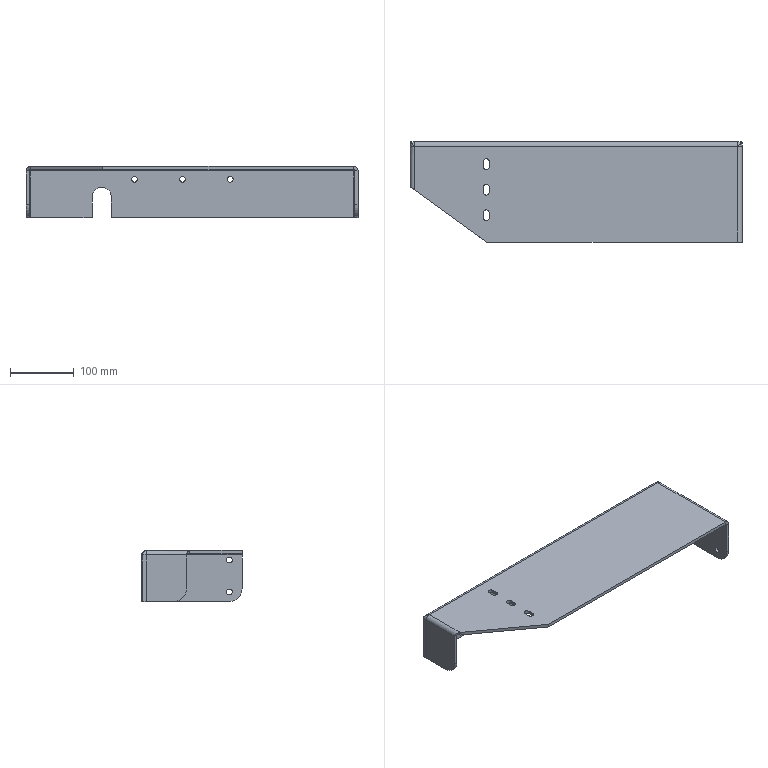Part | SolidWorks | features ICE 3, Cut 2, SMWeldBead 2, EdgeFlange 1, Fillet 1, FlatPattern 1, SMBaseFlange 1, SheetMetal 1 | 1 solid | 78 faces | box 520 x 157 x 80 mm | volume 639490 mm3 | cylinder 40 | plane 35 | spline 3 | commonest cylinder face diameters 9 x20 4 x7 14 x7 2 x2 30 x2 40 x2